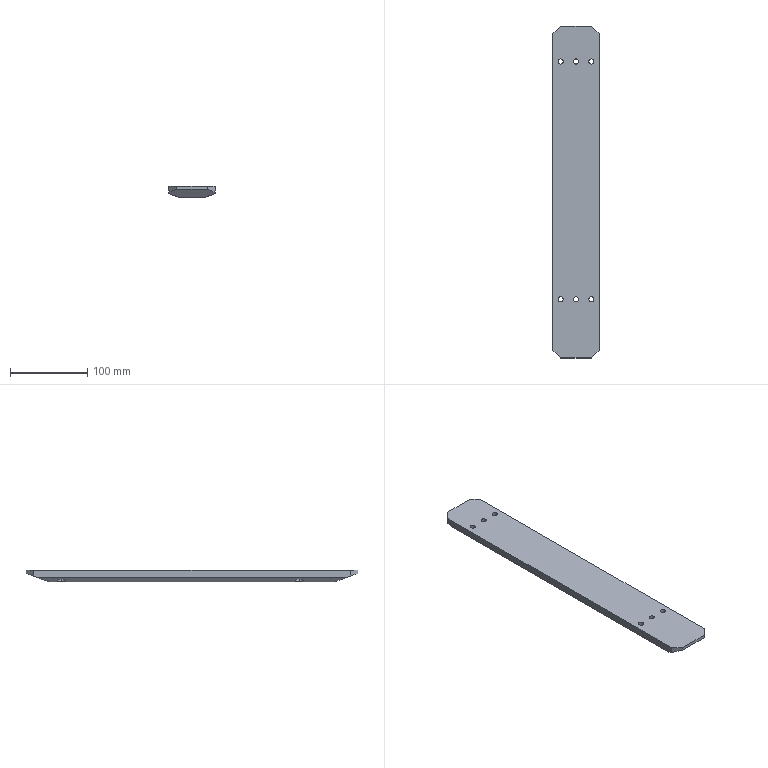Part | SolidWorks | features BaseBody 1 | 1 solid | 44 faces | box 60 x 430 x 15 mm | volume 329496 mm3 | cylinder 24 | plane 20 | commonest cylinder face diameters 6.6 x12 11 x12
STEP:
#1=CARTESIAN_POINT('',(25.5,169.,9.));
#2=VERTEX_POINT('',#1);
#3=CARTESIAN_POINT('',(14.5,169.,9.));
#4=VERTEX_POINT('',#3);
#5=CARTESIAN_POINT('',(20.,169.,9.));
#6=DIRECTION('',(0.,0.,-1.));
#7=DIRECTION('',(-1.,0.,0.));
#8=AXIS2_PLACEMENT_3D('',#5,#6,#7);
#9=CIRCLE('',#8,5.5);
#10=EDGE_CURVE('',#2,#4,#9,.T.);
#11=ORIENTED_EDGE('',*,*,#10,.F.);
#12=CARTESIAN_POINT('',(25.5,169.,3.822));
#13=VERTEX_POINT('',#12);
#14=CARTESIAN_POINT('',(25.5,169.,0.));
#15=DIRECTION('',(0.,0.,-1.));
#16=VECTOR('',#15,1000.);
#17=LINE('',#14,#16);
#18=EDGE_CURVE('',#2,#13,#17,.T.);
#19=ORIENTED_EDGE('',*,*,#18,.T.);
#20=CARTESIAN_POINT('',(15.,166.709,0.));
#21=VERTEX_POINT('',#20);
#22=CARTESIAN_POINT('',(25.5,169.,3.822));
#23=CARTESIAN_POINT('',(25.5,161.466,3.822));
#24=CARTESIAN_POINT('',(18.139,159.859,1.142));
#25=CARTESIAN_POINT('',(15.,166.709,0.));
#26=(BOUNDED_CURVE()B_SPLINE_CURVE(3,(#22,#23,#24,#25),.UNSPECIFIED.,.F.,.F.)B_SPLINE_CURVE_WITH_KNOTS((4,4),(3.142,5.853),.UNSPECIFIED.)CURVE()GEOMETRIC_REPRESENTATION_ITEM()RATIONAL_B_SPLINE_CURVE((1.,0.4755,0.4755,1.))REPRESENTATION_ITEM(''));
#27=EDGE_CURVE('',#13,#21,#26,.T.);
#28=ORIENTED_EDGE('',*,*,#27,.T.);
#29=CARTESIAN_POINT('',(14.5,169.,0.));
#30=VERTEX_POINT('',#29);
#31=CARTESIAN_POINT('',(20.,169.,0.));
#32=DIRECTION('',(0.,0.,-1.));
#33=DIRECTION('',(-1.,0.,0.));
#34=AXIS2_PLACEMENT_3D('',#31,#32,#33);
#35=CIRCLE('',#34,5.5);
#36=EDGE_CURVE('',#21,#30,#35,.T.);
#37=ORIENTED_EDGE('',*,*,#36,.T.);
#38=CARTESIAN_POINT('',(14.5,169.,0.));
#39=DIRECTION('',(0.,0.,-1.));
#40=VECTOR('',#39,1000.);
#41=LINE('',#38,#40);
#42=EDGE_CURVE('',#4,#30,#41,.T.);
#43=ORIENTED_EDGE('',*,*,#42,.F.);
#44=EDGE_LOOP('',(#11,#19,#28,#37,#43));
#45=FACE_OUTER_BOUND('',#44,.T.);
#46=CARTESIAN_POINT('',(20.,169.,0.));
#47=DIRECTION('',(0.,0.,-1.));
#48=DIRECTION('',(-1.,0.,0.));
#49=AXIS2_PLACEMENT_3D('',#46,#47,#48);
#50=CYLINDRICAL_SURFACE('',#49,5.5);
#51=ADVANCED_FACE('',(#45),#50,.F.);
#52=CARTESIAN_POINT('',(23.3,169.,15.));
#53=VERTEX_POINT('',#52);
#54=CARTESIAN_POINT('',(16.7,169.,15.));
#55=VERTEX_POINT('',#54);
#56=CARTESIAN_POINT('',(20.,169.,15.));
#57=DIRECTION('',(0.,0.,-1.));
#58=DIRECTION('',(-1.,0.,0.));
#59=AXIS2_PLACEMENT_3D('',#56,#57,#58);
#60=CIRCLE('',#59,3.3);
#61=EDGE_CURVE('',#53,#55,#60,.T.);
#62=ORIENTED_EDGE('',*,*,#61,.F.);
#63=CARTESIAN_POINT('',(23.3,169.,9.));
#64=VERTEX_POINT('',#63);
#65=CARTESIAN_POINT('',(23.3,169.,0.));
#66=DIRECTION('',(0.,0.,-1.));
#67=VECTOR('',#66,1000.);
#68=LINE('',#65,#67);
#69=EDGE_CURVE('',#53,#64,#68,.T.);
#70=ORIENTED_EDGE('',*,*,#69,.T.);
#71=CARTESIAN_POINT('',(16.7,169.,9.));
#72=VERTEX_POINT('',#71);
#73=CARTESIAN_POINT('',(20.,169.,9.));
#74=DIRECTION('',(0.,0.,-1.));
#75=DIRECTION('',(-1.,0.,0.));
#76=AXIS2_PLACEMENT_3D('',#73,#74,#75);
#77=CIRCLE('',#76,3.3);
#78=EDGE_CURVE('',#64,#72,#77,.T.);
#79=ORIENTED_EDGE('',*,*,#78,.T.);
#80=CARTESIAN_POINT('',(16.7,169.,0.));
#81=DIRECTION('',(0.,0.,-1.));
#82=VECTOR('',#81,1000.);
#83=LINE('',#80,#82);
#84=EDGE_CURVE('',#55,#72,#83,.T.);
#85=ORIENTED_EDGE('',*,*,#84,.F.);
#86=EDGE_LOOP('',(#62,#70,#79,#85));
#87=FACE_OUTER_BOUND('',#86,.T.);
#88=CARTESIAN_POINT('',(20.,169.,0.));
#89=DIRECTION('',(0.,0.,-1.));
#90=DIRECTION('',(-1.,0.,0.));
#91=AXIS2_PLACEMENT_3D('',#88,#89,#90);
#92=CYLINDRICAL_SURFACE('',#91,3.3);
#93=ADVANCED_FACE('',(#87),#92,.F.);
#94=CARTESIAN_POINT('',(5.5,169.,9.));
#95=VERTEX_POINT('',#94);
#96=CARTESIAN_POINT('',(-5.5,169.,9.));
#97=VERTEX_POINT('',#96);
#98=CARTESIAN_POINT('',(0.,169.,9.));
#99=DIRECTION('',(0.,0.,-1.));
#100=DIRECTION('',(-1.,0.,0.));
#101=AXIS2_PLACEMENT_3D('',#98,#99,#100);
#102=CIRCLE('',#101,5.5);
#103=EDGE_CURVE('',#95,#97,#102,.T.);
#104=ORIENTED_EDGE('',*,*,#103,.F.);
#105=CARTESIAN_POINT('',(5.5,169.,0.));
#106=VERTEX_POINT('',#105);
#107=CARTESIAN_POINT('',(5.5,169.,0.));
#108=DIRECTION('',(0.,0.,-1.));
#109=VECTOR('',#108,1000.);
#110=LINE('',#107,#109);
#111=EDGE_CURVE('',#95,#106,#110,.T.);
#112=ORIENTED_EDGE('',*,*,#111,.T.);
#113=CARTESIAN_POINT('',(-5.5,169.,0.));
#114=VERTEX_POINT('',#113);
#115=CARTESIAN_POINT('',(0.,169.,0.));
#116=DIRECTION('',(0.,0.,-1.));
#117=DIRECTION('',(-1.,0.,0.));
#118=AXIS2_PLACEMENT_3D('',#115,#116,#117);
#119=CIRCLE('',#118,5.5);
#120=EDGE_CURVE('',#106,#114,#119,.T.);
#121=ORIENTED_EDGE('',*,*,#120,.T.);
#122=CARTESIAN_POINT('',(-5.5,169.,0.));
#123=DIRECTION('',(0.,0.,-1.));
#124=VECTOR('',#123,1000.);
#125=LINE('',#122,#124);
#126=EDGE_CURVE('',#97,#114,#125,.T.);
#127=ORIENTED_EDGE('',*,*,#126,.F.);
#128=EDGE_LOOP('',(#104,#112,#121,#127));
#129=FACE_OUTER_BOUND('',#128,.T.);
#130=CARTESIAN_POINT('',(0.,169.,0.));
#131=DIRECTION('',(0.,0.,-1.));
#132=DIRECTION('',(-1.,0.,0.));
#133=AXIS2_PLACEMENT_3D('',#130,#131,#132);
#134=CYLINDRICAL_SURFACE('',#133,5.5);
#135=ADVANCED_FACE('',(#129),#134,.F.);
#136=CARTESIAN_POINT('',(3.3,169.,15.));
#137=VERTEX_POINT('',#136);
#138=CARTESIAN_POINT('',(-3.3,169.,15.));
#139=VERTEX_POINT('',#138);
#140=CARTESIAN_POINT('',(0.,169.,15.));
#141=DIRECTION('',(0.,0.,-1.));
#142=DIRECTION('',(-1.,0.,0.));
#143=AXIS2_PLACEMENT_3D('',#140,#141,#142);
#144=CIRCLE('',#143,3.3);
#145=EDGE_CURVE('',#137,#139,#144,.T.);
#146=ORIENTED_EDGE('',*,*,#145,.F.);
#147=CARTESIAN_POINT('',(3.3,169.,9.));
#148=VERTEX_POINT('',#147);
#149=CARTESIAN_POINT('',(3.3,169.,0.));
#150=DIRECTION('',(0.,0.,-1.));
#151=VECTOR('',#150,1000.);
#152=LINE('',#149,#151);
#153=EDGE_CURVE('',#137,#148,#152,.T.);
#154=ORIENTED_EDGE('',*,*,#153,.T.);
#155=CARTESIAN_POINT('',(-3.3,169.,9.));
#156=VERTEX_POINT('',#155);
#157=CARTESIAN_POINT('',(0.,169.,9.));
#158=DIRECTION('',(0.,0.,-1.));
#159=DIRECTION('',(-1.,0.,0.));
#160=AXIS2_PLACEMENT_3D('',#157,#158,#159);
#161=CIRCLE('',#160,3.3);
#162=EDGE_CURVE('',#148,#156,#161,.T.);
#163=ORIENTED_EDGE('',*,*,#162,.T.);
#164=CARTESIAN_POINT('',(-3.3,169.,0.));
#165=DIRECTION('',(0.,0.,-1.));
#166=VECTOR('',#165,1000.);
#167=LINE('',#164,#166);
#168=EDGE_CURVE('',#139,#156,#167,.T.);
#169=ORIENTED_EDGE('',*,*,#168,.F.);
#170=EDGE_LOOP('',(#146,#154,#163,#169));
#171=FACE_OUTER_BOUND('',#170,.T.);
#172=CARTESIAN_POINT('',(0.,169.,0.));
#173=DIRECTION('',(0.,0.,-1.));
#174=DIRECTION('',(-1.,0.,0.));
#175=AXIS2_PLACEMENT_3D('',#172,#173,#174);
#176=CYLINDRICAL_SURFACE('',#175,3.3);
#177=ADVANCED_FACE('',(#171),#176,.F.);
#178=CARTESIAN_POINT('',(-14.5,169.,9.));
#179=VERTEX_POINT('',#178);
#180=CARTESIAN_POINT('',(-25.5,169.,9.));
#181=VERTEX_POINT('',#180);
#182=CARTESIAN_POINT('',(-20.,169.,9.));
#183=DIRECTION('',(0.,0.,-1.));
#184=DIRECTION('',(-1.,0.,0.));
#185=AXIS2_PLACEMENT_3D('',#182,#183,#184);
#186=CIRCLE('',#185,5.5);
#187=EDGE_CURVE('',#179,#181,#186,.T.);
#188=ORIENTED_EDGE('',*,*,#187,.F.);
#189=CARTESIAN_POINT('',(-14.5,169.,0.));
#190=VERTEX_POINT('',#189);
#191=CARTESIAN_POINT('',(-14.5,169.,0.));
#192=DIRECTION('',(0.,0.,-1.));
#193=VECTOR('',#192,1000.);
#194=LINE('',#191,#193);
#195=EDGE_CURVE('',#179,#190,#194,.T.);
#196=ORIENTED_EDGE('',*,*,#195,.T.);
#197=CARTESIAN_POINT('',(-15.,166.709,0.));
#198=VERTEX_POINT('',#197);
#199=CARTESIAN_POINT('',(-20.,169.,0.));
#200=DIRECTION('',(0.,0.,-1.));
#201=DIRECTION('',(-1.,0.,0.));
#202=AXIS2_PLACEMENT_3D('',#199,#200,#201);
#203=CIRCLE('',#202,5.5);
#204=EDGE_CURVE('',#190,#198,#203,.T.);
#205=ORIENTED_EDGE('',*,*,#204,.T.);
#206=CARTESIAN_POINT('',(-25.5,169.,3.822));
#207=VERTEX_POINT('',#206);
#208=CARTESIAN_POINT('',(-15.,166.709,0.));
#209=CARTESIAN_POINT('',(-18.139,159.859,1.142));
#210=CARTESIAN_POINT('',(-25.5,161.466,3.822));
#211=CARTESIAN_POINT('',(-25.5,169.,3.822));
#212=(BOUNDED_CURVE()B_SPLINE_CURVE(3,(#208,#209,#210,#211),.UNSPECIFIED.,.F.,.F.)B_SPLINE_CURVE_WITH_KNOTS((4,4),(0.4297,3.142),.UNSPECIFIED.)CURVE()GEOMETRIC_REPRESENTATION_ITEM()RATIONAL_B_SPLINE_CURVE((1.,0.4755,0.4755,1.))REPRESENTATION_ITEM(''));
#213=EDGE_CURVE('',#198,#207,#212,.T.);
#214=ORIENTED_EDGE('',*,*,#213,.T.);
#215=CARTESIAN_POINT('',(-25.5,169.,0.));
#216=DIRECTION('',(0.,0.,-1.));
#217=VECTOR('',#216,1000.);
#218=LINE('',#215,#217);
#219=EDGE_CURVE('',#181,#207,#218,.T.);
#220=ORIENTED_EDGE('',*,*,#219,.F.);
#221=EDGE_LOOP('',(#188,#196,#205,#214,#220));
#222=FACE_OUTER_BOUND('',#221,.T.);
#223=CARTESIAN_POINT('',(-20.,169.,0.));
#224=DIRECTION('',(0.,0.,-1.));
#225=DIRECTION('',(-1.,0.,0.));
#226=AXIS2_PLACEMENT_3D('',#223,#224,#225);
#227=CYLINDRICAL_SURFACE('',#226,5.5);
#228=ADVANCED_FACE('',(#222),#227,.F.);
#229=CARTESIAN_POINT('',(-16.7,169.,15.));
#230=VERTEX_POINT('',#229);
#231=CARTESIAN_POINT('',(-23.3,169.,15.));
#232=VERTEX_POINT('',#231);
#233=CARTESIAN_POINT('',(-20.,169.,15.));
#234=DIRECTION('',(0.,0.,-1.));
#235=DIRECTION('',(-1.,0.,0.));
#236=AXIS2_PLACEMENT_3D('',#233,#234,#235);
#237=CIRCLE('',#236,3.3);
#238=EDGE_CURVE('',#230,#232,#237,.T.);
#239=ORIENTED_EDGE('',*,*,#238,.F.);
#240=CARTESIAN_POINT('',(-16.7,169.,9.));
#241=VERTEX_POINT('',#240);
#242=CARTESIAN_POINT('',(-16.7,169.,0.));
#243=DIRECTION('',(0.,0.,-1.));
#244=VECTOR('',#243,1000.);
#245=LINE('',#242,#244);
#246=EDGE_CURVE('',#230,#241,#245,.T.);
#247=ORIENTED_EDGE('',*,*,#246,.T.);
#248=CARTESIAN_POINT('',(-23.3,169.,9.));
#249=VERTEX_POINT('',#248);
#250=CARTESIAN_POINT('',(-20.,169.,9.));
#251=DIRECTION('',(0.,0.,-1.));
#252=DIRECTION('',(-1.,0.,0.));
#253=AXIS2_PLACEMENT_3D('',#250,#251,#252);
#254=CIRCLE('',#253,3.3);
#255=EDGE_CURVE('',#241,#249,#254,.T.);
#256=ORIENTED_EDGE('',*,*,#255,.T.);
#257=CARTESIAN_POINT('',(-23.3,169.,0.));
#258=DIRECTION('',(0.,0.,-1.));
#259=VECTOR('',#258,1000.);
#260=LINE('',#257,#259);
#261=EDGE_CURVE('',#232,#249,#260,.T.);
#262=ORIENTED_EDGE('',*,*,#261,.F.);
#263=EDGE_LOOP('',(#239,#247,#256,#262));
#264=FACE_OUTER_BOUND('',#263,.T.);
#265=CARTESIAN_POINT('',(-20.,169.,0.));
#266=DIRECTION('',(0.,0.,-1.));
#267=DIRECTION('',(-1.,0.,0.));
#268=AXIS2_PLACEMENT_3D('',#265,#266,#267);
#269=CYLINDRICAL_SURFACE('',#268,3.3);
#270=ADVANCED_FACE('',(#264),#269,.F.);
#271=CARTESIAN_POINT('',(25.5,-139.,9.));
#272=VERTEX_POINT('',#271);
#273=CARTESIAN_POINT('',(14.5,-139.,9.));
#274=VERTEX_POINT('',#273);
#275=CARTESIAN_POINT('',(20.,-139.,9.));
#276=DIRECTION('',(0.,0.,-1.));
#277=DIRECTION('',(-1.,0.,0.));
#278=AXIS2_PLACEMENT_3D('',#275,#276,#277);
#279=CIRCLE('',#278,5.5);
#280=EDGE_CURVE('',#272,#274,#279,.T.);
#281=ORIENTED_EDGE('',*,*,#280,.F.);
#282=CARTESIAN_POINT('',(25.5,-139.,3.822));
#283=VERTEX_POINT('',#282);
#284=CARTESIAN_POINT('',(25.5,-139.,0.));
#285=DIRECTION('',(0.,0.,-1.));
#286=VECTOR('',#285,1000.);
#287=LINE('',#284,#286);
#288=EDGE_CURVE('',#272,#283,#287,.T.);
#289=ORIENTED_EDGE('',*,*,#288,.T.);
#290=CARTESIAN_POINT('',(15.,-141.291,0.));
#291=VERTEX_POINT('',#290);
#292=CARTESIAN_POINT('',(25.5,-139.,3.822));
#293=CARTESIAN_POINT('',(25.5,-146.534,3.822));
#294=CARTESIAN_POINT('',(18.139,-148.141,1.142));
#295=CARTESIAN_POINT('',(15.,-141.291,0.));
#296=(BOUNDED_CURVE()B_SPLINE_CURVE(3,(#292,#293,#294,#295),.UNSPECIFIED.,.F.,.T.)B_SPLINE_CURVE_WITH_KNOTS((4,4),(3.142,5.853),.UNSPECIFIED.)CURVE()GEOMETRIC_REPRESENTATION_ITEM()RATIONAL_B_SPLINE_CURVE((1.,0.4755,0.4755,1.))REPRESENTATION_ITEM(''));
#297=EDGE_CURVE('',#283,#291,#296,.T.);
#298=ORIENTED_EDGE('',*,*,#297,.T.);
#299=CARTESIAN_POINT('',(14.5,-139.,0.));
#300=VERTEX_POINT('',#299);
#301=CARTESIAN_POINT('',(20.,-139.,0.));
#302=DIRECTION('',(0.,0.,-1.));
#303=DIRECTION('',(-1.,0.,0.));
#304=AXIS2_PLACEMENT_3D('',#301,#302,#303);
#305=CIRCLE('',#304,5.5);
#306=EDGE_CURVE('',#291,#300,#305,.T.);
#307=ORIENTED_EDGE('',*,*,#306,.T.);
#308=CARTESIAN_POINT('',(14.5,-139.,0.));
#309=DIRECTION('',(0.,0.,-1.));
#310=VECTOR('',#309,1000.);
#311=LINE('',#308,#310);
#312=EDGE_CURVE('',#274,#300,#311,.T.);
#313=ORIENTED_EDGE('',*,*,#312,.F.);
#314=EDGE_LOOP('',(#281,#289,#298,#307,#313));
#315=FACE_OUTER_BOUND('',#314,.T.);
#316=CARTESIAN_POINT('',(20.,-139.,0.));
#317=DIRECTION('',(0.,0.,-1.));
#318=DIRECTION('',(-1.,0.,0.));
#319=AXIS2_PLACEMENT_3D('',#316,#317,#318);
#320=CYLINDRICAL_SURFACE('',#319,5.5);
#321=ADVANCED_FACE('',(#315),#320,.F.);
#322=CARTESIAN_POINT('',(23.3,-139.,15.));
#323=VERTEX_POINT('',#322);
#324=CARTESIAN_POINT('',(16.7,-139.,15.));
#325=VERTEX_POINT('',#324);
#326=CARTESIAN_POINT('',(20.,-139.,15.));
#327=DIRECTION('',(0.,0.,-1.));
#328=DIRECTION('',(-1.,0.,0.));
#329=AXIS2_PLACEMENT_3D('',#326,#327,#328);
#330=CIRCLE('',#329,3.3);
#331=EDGE_CURVE('',#323,#325,#330,.T.);
#332=ORIENTED_EDGE('',*,*,#331,.F.);
#333=CARTESIAN_POINT('',(23.3,-139.,9.));
#334=VERTEX_POINT('',#333);
#335=CARTESIAN_POINT('',(23.3,-139.,0.));
#336=DIRECTION('',(0.,0.,-1.));
#337=VECTOR('',#336,1000.);
#338=LINE('',#335,#337);
#339=EDGE_CURVE('',#323,#334,#338,.T.);
#340=ORIENTED_EDGE('',*,*,#339,.T.);
#341=CARTESIAN_POINT('',(16.7,-139.,9.));
#342=VERTEX_POINT('',#341);
#343=CARTESIAN_POINT('',(20.,-139.,9.));
#344=DIRECTION('',(0.,0.,-1.));
#345=DIRECTION('',(-1.,0.,0.));
#346=AXIS2_PLACEMENT_3D('',#343,#344,#345);
#347=CIRCLE('',#346,3.3);
#348=EDGE_CURVE('',#334,#342,#347,.T.);
#349=ORIENTED_EDGE('',*,*,#348,.T.);
#350=CARTESIAN_POINT('',(16.7,-139.,0.));
#351=DIRECTION('',(0.,0.,-1.));
#352=VECTOR('',#351,1000.);
#353=LINE('',#350,#352);
#354=EDGE_CURVE('',#325,#342,#353,.T.);
#355=ORIENTED_EDGE('',*,*,#354,.F.);
#356=EDGE_LOOP('',(#332,#340,#349,#355));
#357=FACE_OUTER_BOUND('',#356,.T.);
#358=CARTESIAN_POINT('',(20.,-139.,0.));
#359=DIRECTION('',(0.,0.,-1.));
#360=DIRECTION('',(-1.,0.,0.));
#361=AXIS2_PLACEMENT_3D('',#358,#359,#360);
#362=CYLINDRICAL_SURFACE('',#361,3.3);
#363=ADVANCED_FACE('',(#357),#362,.F.);
#364=CARTESIAN_POINT('',(5.5,-139.,9.));
#365=VERTEX_POINT('',#364);
#366=CARTESIAN_POINT('',(-5.5,-139.,9.));
#367=VERTEX_POINT('',#366);
#368=CARTESIAN_POINT('',(0.,-139.,9.));
#369=DIRECTION('',(0.,0.,-1.));
#370=DIRECTION('',(-1.,0.,0.));
#371=AXIS2_PLACEMENT_3D('',#368,#369,#370);
#372=CIRCLE('',#371,5.5);
#373=EDGE_CURVE('',#365,#367,#372,.T.);
#374=ORIENTED_EDGE('',*,*,#373,.F.);
#375=CARTESIAN_POINT('',(5.5,-139.,0.));
#376=VERTEX_POINT('',#375);
#377=CARTESIAN_POINT('',(5.5,-139.,0.));
#378=DIRECTION('',(0.,0.,-1.));
#379=VECTOR('',#378,1000.);
#380=LINE('',#377,#379);
#381=EDGE_CURVE('',#365,#376,#380,.T.);
#382=ORIENTED_EDGE('',*,*,#381,.T.);
#383=CARTESIAN_POINT('',(-5.5,-139.,0.));
#384=VERTEX_POINT('',#383);
#385=CARTESIAN_POINT('',(0.,-139.,0.));
#386=DIRECTION('',(0.,0.,-1.));
#387=DIRECTION('',(-1.,0.,0.));
#388=AXIS2_PLACEMENT_3D('',#385,#386,#387);
#389=CIRCLE('',#388,5.5);
#390=EDGE_CURVE('',#376,#384,#389,.T.);
#391=ORIENTED_EDGE('',*,*,#390,.T.);
#392=CARTESIAN_POINT('',(-5.5,-139.,0.));
#393=DIRECTION('',(0.,0.,-1.));
#394=VECTOR('',#393,1000.);
#395=LINE('',#392,#394);
#396=EDGE_CURVE('',#367,#384,#395,.T.);
#397=ORIENTED_EDGE('',*,*,#396,.F.);
#398=EDGE_LOOP('',(#374,#382,#391,#397));
#399=FACE_OUTER_BOUND('',#398,.T.);
#400=CARTESIAN_POINT('',(0.,-139.,0.));
#401=DIRECTION('',(0.,0.,-1.));
#402=DIRECTION('',(-1.,0.,0.));
#403=AXIS2_PLACEMENT_3D('',#400,#401,#402);
#404=CYLINDRICAL_SURFACE('',#403,5.5);
#405=ADVANCED_FACE('',(#399),#404,.F.);
#406=CARTESIAN_POINT('',(3.3,-139.,15.));
#407=VERTEX_POINT('',#406);
#408=CARTESIAN_POINT('',(-3.3,-139.,15.));
#409=VERTEX_POINT('',#408);
#410=CARTESIAN_POINT('',(0.,-139.,15.));
#411=DIRECTION('',(0.,0.,-1.));
#412=DIRECTION('',(-1.,0.,0.));
#413=AXIS2_PLACEMENT_3D('',#410,#411,#412);
#414=CIRCLE('',#413,3.3);
#415=EDGE_CURVE('',#407,#409,#414,.T.);
#416=ORIENTED_EDGE('',*,*,#415,.F.);
#417=CARTESIAN_POINT('',(3.3,-139.,9.));
#418=VERTEX_POINT('',#417);
#419=CARTESIAN_POINT('',(3.3,-139.,0.));
#420=DIRECTION('',(0.,0.,-1.));
#421=VECTOR('',#420,1000.);
#422=LINE('',#419,#421);
#423=EDGE_CURVE('',#407,#418,#422,.T.);
#424=ORIENTED_EDGE('',*,*,#423,.T.);
#425=CARTESIAN_POINT('',(-3.3,-139.,9.));
#426=VERTEX_POINT('',#425);
#427=CARTESIAN_POINT('',(0.,-139.,9.));
#428=DIRECTION('',(0.,0.,-1.));
#429=DIRECTION('',(-1.,0.,0.));
#430=AXIS2_PLACEMENT_3D('',#427,#428,#429);
#431=CIRCLE('',#430,3.3);
#432=EDGE_CURVE('',#418,#426,#431,.T.);
#433=ORIENTED_EDGE('',*,*,#432,.T.);
#434=CARTESIAN_POINT('',(-3.3,-139.,0.));
#435=DIRECTION('',(0.,0.,-1.));
#436=VECTOR('',#435,1000.);
#437=LINE('',#434,#436);
#438=EDGE_CURVE('',#409,#426,#437,.T.);
#439=ORIENTED_EDGE('',*,*,#438,.F.);
#440=EDGE_LOOP('',(#416,#424,#433,#439));
#441=FACE_OUTER_BOUND('',#440,.T.);
#442=CARTESIAN_POINT('',(0.,-139.,0.));
#443=DIRECTION('',(0.,0.,-1.));
#444=DIRECTION('',(-1.,0.,0.));
#445=AXIS2_PLACEMENT_3D('',#442,#443,#444);
#446=CYLINDRICAL_SURFACE('',#445,3.3);
#447=ADVANCED_FACE('',(#441),#446,.F.);
#448=CARTESIAN_POINT('',(-14.5,-139.,9.));
#449=VERTEX_POINT('',#448);
#450=CARTESIAN_POINT('',(-25.5,-139.,9.));
#451=VERTEX_POINT('',#450);
#452=CARTESIAN_POINT('',(-20.,-139.,9.));
#453=DIRECTION('',(0.,0.,-1.));
#454=DIRECTION('',(-1.,0.,0.));
#455=AXIS2_PLACEMENT_3D('',#452,#453,#454);
#456=CIRCLE('',#455,5.5);
#457=EDGE_CURVE('',#449,#451,#456,.T.);
#458=ORIENTED_EDGE('',*,*,#457,.F.);
#459=CARTESIAN_POINT('',(-14.5,-139.,0.));
#460=VERTEX_POINT('',#459);
#461=CARTESIAN_POINT('',(-14.5,-139.,0.));
#462=DIRECTION('',(0.,0.,-1.));
#463=VECTOR('',#462,1000.);
#464=LINE('',#461,#463);
#465=EDGE_CURVE('',#449,#460,#464,.T.);
#466=ORIENTED_EDGE('',*,*,#465,.T.);
#467=CARTESIAN_POINT('',(-15.,-141.291,0.));
#468=VERTEX_POINT('',#467);
#469=CARTESIAN_POINT('',(-20.,-139.,0.));
#470=DIRECTION('',(0.,0.,-1.));
#471=DIRECTION('',(-1.,0.,0.));
#472=AXIS2_PLACEMENT_3D('',#469,#470,#471);
#473=CIRCLE('',#472,5.5);
#474=EDGE_CURVE('',#460,#468,#473,.T.);
#475=ORIENTED_EDGE('',*,*,#474,.T.);
#476=CARTESIAN_POINT('',(-25.5,-139.,3.822));
#477=VERTEX_POINT('',#476);
#478=CARTESIAN_POINT('',(-15.,-141.291,0.));
#479=CARTESIAN_POINT('',(-18.139,-148.141,1.142));
#480=CARTESIAN_POINT('',(-25.5,-146.534,3.822));
#481=CARTESIAN_POINT('',(-25.5,-139.,3.822));
#482=(BOUNDED_CURVE()B_SPLINE_CURVE(3,(#478,#479,#480,#481),.UNSPECIFIED.,.F.,.T.)B_SPLINE_CURVE_WITH_KNOTS((4,4),(0.4297,3.142),.UNSPECIFIED.)CURVE()GEOMETRIC_REPRESENTATION_ITEM()RATIONAL_B_SPLINE_CURVE((1.,0.4755,0.4755,1.))REPRESENTATION_ITEM(''));
#483=EDGE_CURVE('',#468,#477,#482,.T.);
#484=ORIENTED_EDGE('',*,*,#483,.T.);
#485=CARTESIAN_POINT('',(-25.5,-139.,0.));
#486=DIRECTION('',(0.,0.,-1.));
#487=VECTOR('',#486,1000.);
#488=LINE('',#485,#487);
#489=EDGE_CURVE('',#451,#477,#488,.T.);
#490=ORIENTED_EDGE('',*,*,#489,.F.);
#491=EDGE_LOOP('',(#458,#466,#475,#484,#490));
#492=FACE_OUTER_BOUND('',#491,.T.);
#493=CARTESIAN_POINT('',(-20.,-139.,0.));
#494=DIRECTION('',(0.,0.,-1.));
#495=DIRECTION('',(-1.,0.,0.));
#496=AXIS2_PLACEMENT_3D('',#493,#494,#495);
#497=CYLINDRICAL_SURFACE('',#496,5.5);
#498=ADVANCED_FACE('',(#492),#497,.F.);
#499=CARTESIAN_POINT('',(-16.7,-139.,15.));
#500=VERTEX_POINT('',#499);
#501=CARTESIAN_POINT('',(-23.3,-139.,15.));
#502=VERTEX_POINT('',#501);
#503=CARTESIAN_POINT('',(-20.,-139.,15.));
#504=DIRECTION('',(0.,0.,-1.));
#505=DIRECTION('',(-1.,0.,0.));
#506=AXIS2_PLACEMENT_3D('',#503,#504,#505);
#507=CIRCLE('',#506,3.3);
#508=EDGE_CURVE('',#500,#502,#507,.T.);
#509=ORIENTED_EDGE('',*,*,#508,.F.);
#510=CARTESIAN_POINT('',(-16.7,-139.,9.));
#511=VERTEX_POINT('',#510);
#512=CARTESIAN_POINT('',(-16.7,-139.,0.));
#513=DIRECTION('',(0.,0.,-1.));
#514=VECTOR('',#513,1000.);
#515=LINE('',#512,#514);
#516=EDGE_CURVE('',#500,#511,#515,.T.);
#517=ORIENTED_EDGE('',*,*,#516,.T.);
#518=CARTESIAN_POINT('',(-23.3,-139.,9.));
#519=VERTEX_POINT('',#518);
#520=CARTESIAN_POINT('',(-20.,-139.,9.));
#521=DIRECTION('',(0.,0.,-1.));
#522=DIRECTION('',(-1.,0.,0.));
#523=AXIS2_PLACEMENT_3D('',#520,#521,#522);
#524=CIRCLE('',#523,3.3);
#525=EDGE_CURVE('',#511,#519,#524,.T.);
#526=ORIENTED_EDGE('',*,*,#525,.T.);
#527=CARTESIAN_POINT('',(-23.3,-139.,0.));
#528=DIRECTION('',(0.,0.,-1.));
#529=VECTOR('',#528,1000.);
#530=LINE('',#527,#529);
#531=EDGE_CURVE('',#502,#519,#530,.T.);
#532=ORIENTED_EDGE('',*,*,#531,.F.);
#533=EDGE_LOOP('',(#509,#517,#526,#532));
#534=FACE_OUTER_BOUND('',#533,.T.);
#535=CARTESIAN_POINT('',(-20.,-139.,0.));
#536=DIRECTION('',(0.,0.,-1.));
#537=DIRECTION('',(-1.,0.,0.));
#538=AXIS2_PLACEMENT_3D('',#535,#536,#537);
#539=CYLINDRICAL_SURFACE('',#538,3.3);
#540=ADVANCED_FACE('',(#534),#539,.F.);
#541=CARTESIAN_POINT('',(30.,-205.,7.279));
#542=VERTEX_POINT('',#541);
#543=CARTESIAN_POINT('',(30.,-200.,5.46));
#544=VERTEX_POINT('',#543);
#545=CARTESIAN_POINT('',(30.,-215.,10.919));
#546=DIRECTION('',(0.,0.9397,-0.342));
#547=VECTOR('',#546,1000.);
#548=LINE('',#545,#547);
#549=EDGE_CURVE('',#542,#544,#548,.T.);
#550=ORIENTED_EDGE('',*,*,#549,.T.);
#551=CARTESIAN_POINT('',(30.,200.,5.46));
#552=VERTEX_POINT('',#551);
#553=CARTESIAN_POINT('',(30.,215.,5.46));
#554=DIRECTION('',(0.,1.,0.));
#555=VECTOR('',#554,1000.);
#556=LINE('',#553,#555);
#557=EDGE_CURVE('',#544,#552,#556,.T.);
#558=ORIENTED_EDGE('',*,*,#557,.T.);
#559=CARTESIAN_POINT('',(30.,205.,7.279));
#560=VERTEX_POINT('',#559);
#561=CARTESIAN_POINT('',(30.,215.,10.919));
#562=DIRECTION('',(0.,0.9397,0.342));
#563=VECTOR('',#562,1000.);
#564=LINE('',#561,#563);
#565=EDGE_CURVE('',#552,#560,#564,.T.);
#566=ORIENTED_EDGE('',*,*,#565,.T.);
#567=CARTESIAN_POINT('',(30.,205.,15.));
#568=VERTEX_POINT('',#567);
#569=CARTESIAN_POINT('',(30.,205.,15.));
#570=DIRECTION('',(0.,0.,1.));
#571=VECTOR('',#570,1000.);
#572=LINE('',#569,#571);
#573=EDGE_CURVE('',#560,#568,#572,.T.);
#574=ORIENTED_EDGE('',*,*,#573,.T.);
#575=CARTESIAN_POINT('',(30.,-205.,15.));
#576=VERTEX_POINT('',#575);
#577=CARTESIAN_POINT('',(30.,215.,15.));
#578=DIRECTION('',(0.,1.,0.));
#579=VECTOR('',#578,1000.);
#580=LINE('',#577,#579);
#581=EDGE_CURVE('',#576,#568,#580,.T.);
#582=ORIENTED_EDGE('',*,*,#581,.F.);
#583=CARTESIAN_POINT('',(30.,-205.,15.));
#584=DIRECTION('',(0.,0.,-1.));
#585=VECTOR('',#584,1000.);
#586=LINE('',#583,#585);
#587=EDGE_CURVE('',#576,#542,#586,.T.);
#588=ORIENTED_EDGE('',*,*,#587,.T.);
#589=EDGE_LOOP('',(#550,#558,#566,#574,#582,#588));
#590=FACE_OUTER_BOUND('',#589,.T.);
#591=CARTESIAN_POINT('',(30.,215.,15.));
#592=DIRECTION('',(-1.,0.,0.));
#593=DIRECTION('',(0.,-1.,0.));
#594=AXIS2_PLACEMENT_3D('',#591,#592,#593);
#595=PLANE('',#594);
#596=ADVANCED_FACE('',(#590),#595,.F.);
#597=CARTESIAN_POINT('',(20.,215.,15.));
#598=VERTEX_POINT('',#597);
#599=CARTESIAN_POINT('',(20.,215.,10.919));
#600=VERTEX_POINT('',#599);
#601=CARTESIAN_POINT('',(20.,215.,15.));
#602=DIRECTION('',(0.,0.,-1.));
#603=VECTOR('',#602,1000.);
#604=LINE('',#601,#603);
#605=EDGE_CURVE('',#598,#600,#604,.T.);
#606=ORIENTED_EDGE('',*,*,#605,.T.);
#607=CARTESIAN_POINT('',(-20.,215.,10.919));
#608=VERTEX_POINT('',#607);
#609=CARTESIAN_POINT('',(-30.,215.,10.919));
#610=DIRECTION('',(-1.,0.,0.));
#611=VECTOR('',#610,1000.);
#612=LINE('',#609,#611);
#613=EDGE_CURVE('',#600,#608,#612,.T.);
#614=ORIENTED_EDGE('',*,*,#613,.T.);
#615=CARTESIAN_POINT('',(-20.,215.,15.));
#616=VERTEX_POINT('',#615);
#617=CARTESIAN_POINT('',(-20.,215.,15.));
#618=DIRECTION('',(0.,0.,1.));
#619=VECTOR('',#618,1000.);
#620=LINE('',#617,#619);
#621=EDGE_CURVE('',#608,#616,#620,.T.);
#622=ORIENTED_EDGE('',*,*,#621,.T.);
#623=CARTESIAN_POINT('',(-30.,215.,15.));
#624=DIRECTION('',(-1.,0.,0.));
#625=VECTOR('',#624,1000.);
#626=LINE('',#623,#625);
#627=EDGE_CURVE('',#598,#616,#626,.T.);
#628=ORIENTED_EDGE('',*,*,#627,.F.);
#629=EDGE_LOOP('',(#606,#614,#622,#628));
#630=FACE_OUTER_BOUND('',#629,.T.);
#631=CARTESIAN_POINT('',(-30.,215.,15.));
#632=DIRECTION('',(0.,-1.,0.));
#633=DIRECTION('',(0.,0.,-1.));
#634=AXIS2_PLACEMENT_3D('',#631,#632,#633);
#635=PLANE('',#634);
#636=ADVANCED_FACE('',(#630),#635,.F.);
#637=CARTESIAN_POINT('',(-30.,205.,7.279));
#638=VERTEX_POINT('',#637);
#639=CARTESIAN_POINT('',(-30.,200.,5.46));
#640=VERTEX_POINT('',#639);
#641=CARTESIAN_POINT('',(-30.,215.,10.919));
#642=DIRECTION('',(0.,-0.9397,-0.342));
#643=VECTOR('',#642,1000.);
#644=LINE('',#641,#643);
#645=EDGE_CURVE('',#638,#640,#644,.T.);
#646=ORIENTED_EDGE('',*,*,#645,.T.);
#647=CARTESIAN_POINT('',(-30.,-200.,5.46));
#648=VERTEX_POINT('',#647);
#649=CARTESIAN_POINT('',(-30.,215.,5.46));
#650=DIRECTION('',(0.,-1.,0.));
#651=VECTOR('',#650,1000.);
#652=LINE('',#649,#651);
#653=EDGE_CURVE('',#640,#648,#652,.T.);
#654=ORIENTED_EDGE('',*,*,#653,.T.);
#655=CARTESIAN_POINT('',(-30.,-205.,7.279));
#656=VERTEX_POINT('',#655);
#657=CARTESIAN_POINT('',(-30.,-215.,10.919));
#658=DIRECTION('',(0.,-0.9397,0.342));
#659=VECTOR('',#658,1000.);
#660=LINE('',#657,#659);
#661=EDGE_CURVE('',#648,#656,#660,.T.);
#662=ORIENTED_EDGE('',*,*,#661,.T.);
#663=CARTESIAN_POINT('',(-30.,-205.,15.));
#664=VERTEX_POINT('',#663);
#665=CARTESIAN_POINT('',(-30.,-205.,15.));
#666=DIRECTION('',(0.,0.,1.));
#667=VECTOR('',#666,1000.);
#668=LINE('',#665,#667);
#669=EDGE_CURVE('',#656,#664,#668,.T.);
#670=ORIENTED_EDGE('',*,*,#669,.T.);
#671=CARTESIAN_POINT('',(-30.,205.,15.));
#672=VERTEX_POINT('',#671);
#673=CARTESIAN_POINT('',(-30.,215.,15.));
#674=DIRECTION('',(0.,-1.,0.));
#675=VECTOR('',#674,1000.);
#676=LINE('',#673,#675);
#677=EDGE_CURVE('',#672,#664,#676,.T.);
#678=ORIENTED_EDGE('',*,*,#677,.F.);
#679=CARTESIAN_POINT('',(-30.,205.,15.));
#680=DIRECTION('',(0.,0.,-1.));
#681=VECTOR('',#680,1000.);
#682=LINE('',#679,#681);
#683=EDGE_CURVE('',#672,#638,#682,.T.);
#684=ORIENTED_EDGE('',*,*,#683,.T.);
#685=EDGE_LOOP('',(#646,#654,#662,#670,#678,#684));
#686=FACE_OUTER_BOUND('',#685,.T.);
#687=CARTESIAN_POINT('',(-30.,215.,15.));
#688=DIRECTION('',(1.,0.,0.));
#689=DIRECTION('',(0.,1.,0.));
#690=AXIS2_PLACEMENT_3D('',#687,#688,#689);
#691=PLANE('',#690);
#692=ADVANCED_FACE('',(#686),#691,.F.);
#693=CARTESIAN_POINT('',(-20.,-215.,15.));
#694=VERTEX_POINT('',#693);
#695=CARTESIAN_POINT('',(-20.,-215.,10.919));
#696=VERTEX_POINT('',#695);
#697=CARTESIAN_POINT('',(-20.,-215.,15.));
#698=DIRECTION('',(0.,0.,-1.));
#699=VECTOR('',#698,1000.);
#700=LINE('',#697,#699);
#701=EDGE_CURVE('',#694,#696,#700,.T.);
#702=ORIENTED_EDGE('',*,*,#701,.T.);
#703=CARTESIAN_POINT('',(20.,-215.,10.919));
#704=VERTEX_POINT('',#703);
#705=CARTESIAN_POINT('',(-30.,-215.,10.919));
#706=DIRECTION('',(1.,0.,0.));
#707=VECTOR('',#706,1000.);
#708=LINE('',#705,#707);
#709=EDGE_CURVE('',#696,#704,#708,.T.);
#710=ORIENTED_EDGE('',*,*,#709,.T.);
#711=CARTESIAN_POINT('',(20.,-215.,15.));
#712=VERTEX_POINT('',#711);
#713=CARTESIAN_POINT('',(20.,-215.,15.));
#714=DIRECTION('',(0.,0.,1.));
#715=VECTOR('',#714,1000.);
#716=LINE('',#713,#715);
#717=EDGE_CURVE('',#704,#712,#716,.T.);
#718=ORIENTED_EDGE('',*,*,#717,.T.);
#719=CARTESIAN_POINT('',(-30.,-215.,15.));
#720=DIRECTION('',(1.,0.,0.));
#721=VECTOR('',#720,1000.);
#722=LINE('',#719,#721);
#723=EDGE_CURVE('',#694,#712,#722,.T.);
#724=ORIENTED_EDGE('',*,*,#723,.F.);
#725=EDGE_LOOP('',(#702,#710,#718,#724));
#726=FACE_OUTER_BOUND('',#725,.T.);
#727=CARTESIAN_POINT('',(-30.,-215.,15.));
#728=DIRECTION('',(0.,1.,0.));
#729=DIRECTION('',(0.,0.,1.));
#730=AXIS2_PLACEMENT_3D('',#727,#728,#729);
#731=PLANE('',#730);
#732=ADVANCED_FACE('',(#726),#731,.F.);
#733=CARTESIAN_POINT('',(20.,169.,15.));
#734=DIRECTION('',(0.,0.,-1.));
#735=DIRECTION('',(-1.,0.,0.));
#736=AXIS2_PLACEMENT_3D('',#733,#734,#735);
#737=CIRCLE('',#736,3.3);
#738=EDGE_CURVE('',#55,#53,#737,.T.);
#739=ORIENTED_EDGE('',*,*,#738,.T.);
#740=ORIENTED_EDGE('',*,*,#61,.T.);
#741=EDGE_LOOP('',(#739,#740));
#742=FACE_BOUND('',#741,.T.);
#743=CARTESIAN_POINT('',(0.,169.,15.));
#744=DIRECTION('',(0.,0.,-1.));
#745=DIRECTION('',(-1.,0.,0.));
#746=AXIS2_PLACEMENT_3D('',#743,#744,#745);
#747=CIRCLE('',#746,3.3);
#748=EDGE_CURVE('',#139,#137,#747,.T.);
#749=ORIENTED_EDGE('',*,*,#748,.T.);
#750=ORIENTED_EDGE('',*,*,#145,.T.);
#751=EDGE_LOOP('',(#749,#750));
#752=FACE_BOUND('',#751,.T.);
#753=CARTESIAN_POINT('',(-20.,169.,15.));
#754=DIRECTION('',(0.,0.,-1.));
#755=DIRECTION('',(-1.,0.,0.));
#756=AXIS2_PLACEMENT_3D('',#753,#754,#755);
#757=CIRCLE('',#756,3.3);
#758=EDGE_CURVE('',#232,#230,#757,.T.);
#759=ORIENTED_EDGE('',*,*,#758,.T.);
#760=ORIENTED_EDGE('',*,*,#238,.T.);
#761=EDGE_LOOP('',(#759,#760));
#762=FACE_BOUND('',#761,.T.);
#763=CARTESIAN_POINT('',(20.,-139.,15.));
#764=DIRECTION('',(0.,0.,-1.));
#765=DIRECTION('',(-1.,0.,0.));
#766=AXIS2_PLACEMENT_3D('',#763,#764,#765);
#767=CIRCLE('',#766,3.3);
#768=EDGE_CURVE('',#325,#323,#767,.T.);
#769=ORIENTED_EDGE('',*,*,#768,.T.);
#770=ORIENTED_EDGE('',*,*,#331,.T.);
#771=EDGE_LOOP('',(#769,#770));
#772=FACE_BOUND('',#771,.T.);
#773=CARTESIAN_POINT('',(0.,-139.,15.));
#774=DIRECTION('',(0.,0.,-1.));
#775=DIRECTION('',(-1.,0.,0.));
#776=AXIS2_PLACEMENT_3D('',#773,#774,#775);
#777=CIRCLE('',#776,3.3);
#778=EDGE_CURVE('',#409,#407,#777,.T.);
#779=ORIENTED_EDGE('',*,*,#778,.T.);
#780=ORIENTED_EDGE('',*,*,#415,.T.);
#781=EDGE_LOOP('',(#779,#780));
#782=FACE_BOUND('',#781,.T.);
#783=CARTESIAN_POINT('',(-20.,-139.,15.));
#784=DIRECTION('',(0.,0.,-1.));
#785=DIRECTION('',(-1.,0.,0.));
#786=AXIS2_PLACEMENT_3D('',#783,#784,#785);
#787=CIRCLE('',#786,3.3);
#788=EDGE_CURVE('',#502,#500,#787,.T.);
#789=ORIENTED_EDGE('',*,*,#788,.T.);
#790=ORIENTED_EDGE('',*,*,#508,.T.);
#791=EDGE_LOOP('',(#789,#790));
#792=FACE_BOUND('',#791,.T.);
#793=ORIENTED_EDGE('',*,*,#723,.T.);
#794=CARTESIAN_POINT('',(117.5,-117.5,15.));
#795=DIRECTION('',(0.7071,0.7071,0.));
#796=VECTOR('',#795,1000.);
#797=LINE('',#794,#796);
#798=EDGE_CURVE('',#712,#576,#797,.T.);
#799=ORIENTED_EDGE('',*,*,#798,.T.);
#800=ORIENTED_EDGE('',*,*,#581,.T.);
#801=CARTESIAN_POINT('',(117.5,117.5,15.));
#802=DIRECTION('',(-0.7071,0.7071,0.));
#803=VECTOR('',#802,1000.);
#804=LINE('',#801,#803);
#805=EDGE_CURVE('',#568,#598,#804,.T.);
#806=ORIENTED_EDGE('',*,*,#805,.T.);
#807=ORIENTED_EDGE('',*,*,#627,.T.);
#808=CARTESIAN_POINT('',(-117.5,117.5,15.));
#809=DIRECTION('',(-0.7071,-0.7071,0.));
#810=VECTOR('',#809,1000.);
#811=LINE('',#808,#810);
#812=EDGE_CURVE('',#616,#672,#811,.T.);
#813=ORIENTED_EDGE('',*,*,#812,.T.);
#814=ORIENTED_EDGE('',*,*,#677,.T.);
#815=CARTESIAN_POINT('',(-117.5,-117.5,15.));
#816=DIRECTION('',(0.7071,-0.7071,0.));
#817=VECTOR('',#816,1000.);
#818=LINE('',#815,#817);
#819=EDGE_CURVE('',#664,#694,#818,.T.);
#820=ORIENTED_EDGE('',*,*,#819,.T.);
#821=EDGE_LOOP('',(#793,#799,#800,#806,#807,#813,#814,#820));
#822=FACE_OUTER_BOUND('',#821,.T.);
#823=CARTESIAN_POINT('',(0.,0.,15.));
#824=DIRECTION('',(0.,0.,1.));
#825=DIRECTION('',(1.,0.,0.));
#826=AXIS2_PLACEMENT_3D('',#823,#824,#825);
#827=PLANE('',#826);
#828=ADVANCED_FACE('',(#742,#752,#762,#772,#782,#792,#822),#827,.T.);
#829=CARTESIAN_POINT('',(0.,169.,0.));
#830=DIRECTION('',(0.,0.,-1.));
#831=DIRECTION('',(-1.,0.,0.));
#832=AXIS2_PLACEMENT_3D('',#829,#830,#831);
#833=CIRCLE('',#832,5.5);
#834=EDGE_CURVE('',#114,#106,#833,.T.);
#835=ORIENTED_EDGE('',*,*,#834,.F.);
#836=ORIENTED_EDGE('',*,*,#120,.F.);
#837=EDGE_LOOP('',(#835,#836));
#838=FACE_BOUND('',#837,.T.);
#839=CARTESIAN_POINT('',(0.,-139.,0.));
#840=DIRECTION('',(0.,0.,-1.));
#841=DIRECTION('',(-1.,0.,0.));
#842=AXIS2_PLACEMENT_3D('',#839,#840,#841);
#843=CIRCLE('',#842,5.5);
#844=EDGE_CURVE('',#384,#376,#843,.T.);
#845=ORIENTED_EDGE('',*,*,#844,.F.);
#846=ORIENTED_EDGE('',*,*,#390,.F.);
#847=EDGE_LOOP('',(#845,#846));
#848=FACE_BOUND('',#847,.T.);
#849=CARTESIAN_POINT('',(15.,185.,0.));
#850=VERTEX_POINT('',#849);
#851=CARTESIAN_POINT('',(15.,171.291,0.));
#852=VERTEX_POINT('',#851);
#853=CARTESIAN_POINT('',(15.,0.,0.));
#854=DIRECTION('',(0.,-1.,0.));
#855=VECTOR('',#854,1000.);
#856=LINE('',#853,#855);
#857=EDGE_CURVE('',#850,#852,#856,.T.);
#858=ORIENTED_EDGE('',*,*,#857,.T.);
#859=CARTESIAN_POINT('',(20.,169.,0.));
#860=DIRECTION('',(0.,0.,-1.));
#861=DIRECTION('',(-1.,0.,0.));
#862=AXIS2_PLACEMENT_3D('',#859,#860,#861);
#863=CIRCLE('',#862,5.5);
#864=EDGE_CURVE('',#30,#852,#863,.T.);
#865=ORIENTED_EDGE('',*,*,#864,.F.);
#866=ORIENTED_EDGE('',*,*,#36,.F.);
#867=CARTESIAN_POINT('',(15.,-136.709,0.));
#868=VERTEX_POINT('',#867);
#869=CARTESIAN_POINT('',(15.,0.,0.));
#870=DIRECTION('',(0.,-1.,0.));
#871=VECTOR('',#870,1000.);
#872=LINE('',#869,#871);
#873=EDGE_CURVE('',#21,#868,#872,.T.);
#874=ORIENTED_EDGE('',*,*,#873,.T.);
#875=CARTESIAN_POINT('',(20.,-139.,0.));
#876=DIRECTION('',(0.,0.,-1.));
#877=DIRECTION('',(-1.,0.,0.));
#878=AXIS2_PLACEMENT_3D('',#875,#876,#877);
#879=CIRCLE('',#878,5.5);
#880=EDGE_CURVE('',#300,#868,#879,.T.);
#881=ORIENTED_EDGE('',*,*,#880,.F.);
#882=ORIENTED_EDGE('',*,*,#306,.F.);
#883=CARTESIAN_POINT('',(15.,-185.,0.));
#884=VERTEX_POINT('',#883);
#885=CARTESIAN_POINT('',(15.,0.,0.));
#886=DIRECTION('',(0.,-1.,0.));
#887=VECTOR('',#886,1000.);
#888=LINE('',#885,#887);
#889=EDGE_CURVE('',#291,#884,#888,.T.);
#890=ORIENTED_EDGE('',*,*,#889,.T.);
#891=CARTESIAN_POINT('',(-15.,-185.,0.));
#892=VERTEX_POINT('',#891);
#893=CARTESIAN_POINT('',(0.,-185.,0.));
#894=DIRECTION('',(-1.,0.,0.));
#895=VECTOR('',#894,1000.);
#896=LINE('',#893,#895);
#897=EDGE_CURVE('',#884,#892,#896,.T.);
#898=ORIENTED_EDGE('',*,*,#897,.T.);
#899=CARTESIAN_POINT('',(-15.,0.,0.));
#900=DIRECTION('',(0.,1.,0.));
#901=VECTOR('',#900,1000.);
#902=LINE('',#899,#901);
#903=EDGE_CURVE('',#892,#468,#902,.T.);
#904=ORIENTED_EDGE('',*,*,#903,.T.);
#905=ORIENTED_EDGE('',*,*,#474,.F.);
#906=CARTESIAN_POINT('',(-15.,-136.709,0.));
#907=VERTEX_POINT('',#906);
#908=CARTESIAN_POINT('',(-20.,-139.,0.));
#909=DIRECTION('',(0.,0.,-1.));
#910=DIRECTION('',(-1.,0.,0.));
#911=AXIS2_PLACEMENT_3D('',#908,#909,#910);
#912=CIRCLE('',#911,5.5);
#913=EDGE_CURVE('',#907,#460,#912,.T.);
#914=ORIENTED_EDGE('',*,*,#913,.F.);
#915=CARTESIAN_POINT('',(-15.,0.,0.));
#916=DIRECTION('',(0.,1.,0.));
#917=VECTOR('',#916,1000.);
#918=LINE('',#915,#917);
#919=EDGE_CURVE('',#907,#198,#918,.T.);
#920=ORIENTED_EDGE('',*,*,#919,.T.);
#921=ORIENTED_EDGE('',*,*,#204,.F.);
#922=CARTESIAN_POINT('',(-15.,171.291,0.));
#923=VERTEX_POINT('',#922);
#924=CARTESIAN_POINT('',(-20.,169.,0.));
#925=DIRECTION('',(0.,0.,-1.));
#926=DIRECTION('',(-1.,0.,0.));
#927=AXIS2_PLACEMENT_3D('',#924,#925,#926);
#928=CIRCLE('',#927,5.5);
#929=EDGE_CURVE('',#923,#190,#928,.T.);
#930=ORIENTED_EDGE('',*,*,#929,.F.);
#931=CARTESIAN_POINT('',(-15.,185.,0.));
#932=VERTEX_POINT('',#931);
#933=CARTESIAN_POINT('',(-15.,0.,0.));
#934=DIRECTION('',(0.,1.,0.));
#935=VECTOR('',#934,1000.);
#936=LINE('',#933,#935);
#937=EDGE_CURVE('',#923,#932,#936,.T.);
#938=ORIENTED_EDGE('',*,*,#937,.T.);
#939=CARTESIAN_POINT('',(0.,185.,0.));
#940=DIRECTION('',(1.,0.,0.));
#941=VECTOR('',#940,1000.);
#942=LINE('',#939,#941);
#943=EDGE_CURVE('',#932,#850,#942,.T.);
#944=ORIENTED_EDGE('',*,*,#943,.T.);
#945=EDGE_LOOP('',(#858,#865,#866,#874,#881,#882,#890,#898,#904,#905,#914,#920,#921,#930,#938,#944));
#946=FACE_OUTER_BOUND('',#945,.T.);
#947=CARTESIAN_POINT('',(0.,0.,0.));
#948=DIRECTION('',(0.,0.,1.));
#949=DIRECTION('',(1.,0.,0.));
#950=AXIS2_PLACEMENT_3D('',#947,#948,#949);
#951=PLANE('',#950);
#952=ADVANCED_FACE('',(#838,#848,#946),#951,.F.);
#953=ORIENTED_EDGE('',*,*,#717,.F.);
#954=CARTESIAN_POINT('',(28.682,-206.318,7.759));
#955=DIRECTION('',(0.6848,0.6848,-0.2492));
#956=VECTOR('',#955,1000.);
#957=LINE('',#954,#956);
#958=EDGE_CURVE('',#704,#542,#957,.T.);
#959=ORIENTED_EDGE('',*,*,#958,.T.);
#960=ORIENTED_EDGE('',*,*,#587,.F.);
#961=ORIENTED_EDGE('',*,*,#798,.F.);
#962=EDGE_LOOP('',(#953,#959,#960,#961));
#963=FACE_OUTER_BOUND('',#962,.T.);
#964=CARTESIAN_POINT('',(30.,-205.,15.));
#965=DIRECTION('',(-0.7071,0.7071,0.));
#966=DIRECTION('',(0.,0.,-1.));
#967=AXIS2_PLACEMENT_3D('',#964,#965,#966);
#968=PLANE('',#967);
#969=ADVANCED_FACE('',(#963),#968,.F.);
#970=ORIENTED_EDGE('',*,*,#669,.F.);
#971=CARTESIAN_POINT('',(-19.303,-215.697,11.173));
#972=DIRECTION('',(0.6848,-0.6848,0.2492));
#973=VECTOR('',#972,1000.);
#974=LINE('',#971,#973);
#975=EDGE_CURVE('',#656,#696,#974,.T.);
#976=ORIENTED_EDGE('',*,*,#975,.T.);
#977=ORIENTED_EDGE('',*,*,#701,.F.);
#978=ORIENTED_EDGE('',*,*,#819,.F.);
#979=EDGE_LOOP('',(#970,#976,#977,#978));
#980=FACE_OUTER_BOUND('',#979,.T.);
#981=CARTESIAN_POINT('',(-20.,-215.,15.));
#982=DIRECTION('',(0.7071,0.7071,0.));
#983=DIRECTION('',(0.,0.,-1.));
#984=AXIS2_PLACEMENT_3D('',#981,#982,#983);
#985=PLANE('',#984);
#986=ADVANCED_FACE('',(#980),#985,.F.);
#987=ORIENTED_EDGE('',*,*,#573,.F.);
#988=CARTESIAN_POINT('',(19.303,215.697,11.173));
#989=DIRECTION('',(-0.6848,0.6848,0.2492));
#990=VECTOR('',#989,1000.);
#991=LINE('',#988,#990);
#992=EDGE_CURVE('',#560,#600,#991,.T.);
#993=ORIENTED_EDGE('',*,*,#992,.T.);
#994=ORIENTED_EDGE('',*,*,#605,.F.);
#995=ORIENTED_EDGE('',*,*,#805,.F.);
#996=EDGE_LOOP('',(#987,#993,#994,#995));
#997=FACE_OUTER_BOUND('',#996,.T.);
#998=CARTESIAN_POINT('',(20.,215.,15.));
#999=DIRECTION('',(-0.7071,-0.7071,0.));
#1000=DIRECTION('',(0.,0.,-1.));
#1001=AXIS2_PLACEMENT_3D('',#998,#999,#1000);
#1002=PLANE('',#1001);
#1003=ADVANCED_FACE('',(#997),#1002,.F.);
#1004=ORIENTED_EDGE('',*,*,#621,.F.);
#1005=CARTESIAN_POINT('',(-28.682,206.318,7.759));
#1006=DIRECTION('',(-0.6848,-0.6848,-0.2492));
#1007=VECTOR('',#1006,1000.);
#1008=LINE('',#1005,#1007);
#1009=EDGE_CURVE('',#608,#638,#1008,.T.);
#1010=ORIENTED_EDGE('',*,*,#1009,.T.);
#1011=ORIENTED_EDGE('',*,*,#683,.F.);
#1012=ORIENTED_EDGE('',*,*,#812,.F.);
#1013=EDGE_LOOP('',(#1004,#1010,#1011,#1012));
#1014=FACE_OUTER_BOUND('',#1013,.T.);
#1015=CARTESIAN_POINT('',(-30.,205.,15.));
#1016=DIRECTION('',(0.7071,-0.7071,0.));
#1017=DIRECTION('',(0.,0.,-1.));
#1018=AXIS2_PLACEMENT_3D('',#1015,#1016,#1017);
#1019=PLANE('',#1018);
#1020=ADVANCED_FACE('',(#1014),#1019,.F.);
#1021=ORIENTED_EDGE('',*,*,#943,.F.);
#1022=CARTESIAN_POINT('',(-37.966,207.966,8.359));
#1023=DIRECTION('',(-0.6848,0.6848,0.2492));
#1024=VECTOR('',#1023,1000.);
#1025=LINE('',#1022,#1024);
#1026=EDGE_CURVE('',#932,#640,#1025,.T.);
#1027=ORIENTED_EDGE('',*,*,#1026,.T.);
#1028=ORIENTED_EDGE('',*,*,#645,.F.);
#1029=ORIENTED_EDGE('',*,*,#1009,.F.);
#1030=ORIENTED_EDGE('',*,*,#613,.F.);
#1031=ORIENTED_EDGE('',*,*,#992,.F.);
#1032=ORIENTED_EDGE('',*,*,#565,.F.);
#1033=CARTESIAN_POINT('',(9.83,179.83,-1.882));
#1034=DIRECTION('',(-0.6848,-0.6848,-0.2492));
#1035=VECTOR('',#1034,1000.);
#1036=LINE('',#1033,#1035);
#1037=EDGE_CURVE('',#552,#850,#1036,.T.);
#1038=ORIENTED_EDGE('',*,*,#1037,.T.);
#1039=EDGE_LOOP('',(#1021,#1027,#1028,#1029,#1030,#1031,#1032,#1038));
#1040=FACE_OUTER_BOUND('',#1039,.T.);
#1041=CARTESIAN_POINT('',(-30.,215.,10.919));
#1042=DIRECTION('',(0.,-0.342,0.9397));
#1043=DIRECTION('',(-1.,0.,0.));
#1044=AXIS2_PLACEMENT_3D('',#1041,#1042,#1043);
#1045=PLANE('',#1044);
#1046=ADVANCED_FACE('',(#1040),#1045,.F.);
#1047=ORIENTED_EDGE('',*,*,#661,.F.);
#1048=CARTESIAN_POINT('',(-37.966,-207.966,8.359));
#1049=DIRECTION('',(0.6848,0.6848,-0.2492));
#1050=VECTOR('',#1049,1000.);
#1051=LINE('',#1048,#1050);
#1052=EDGE_CURVE('',#648,#892,#1051,.T.);
#1053=ORIENTED_EDGE('',*,*,#1052,.T.);
#1054=ORIENTED_EDGE('',*,*,#897,.F.);
#1055=CARTESIAN_POINT('',(9.83,-179.83,-1.882));
#1056=DIRECTION('',(0.6848,-0.6848,0.2492));
#1057=VECTOR('',#1056,1000.);
#1058=LINE('',#1055,#1057);
#1059=EDGE_CURVE('',#884,#544,#1058,.T.);
#1060=ORIENTED_EDGE('',*,*,#1059,.T.);
#1061=ORIENTED_EDGE('',*,*,#549,.F.);
#1062=ORIENTED_EDGE('',*,*,#958,.F.);
#1063=ORIENTED_EDGE('',*,*,#709,.F.);
#1064=ORIENTED_EDGE('',*,*,#975,.F.);
#1065=EDGE_LOOP('',(#1047,#1053,#1054,#1060,#1061,#1062,#1063,#1064));
#1066=FACE_OUTER_BOUND('',#1065,.T.);
#1067=CARTESIAN_POINT('',(-30.,-215.,10.919));
#1068=DIRECTION('',(0.,0.342,0.9397));
#1069=DIRECTION('',(1.,0.,0.));
#1070=AXIS2_PLACEMENT_3D('',#1067,#1068,#1069);
#1071=PLANE('',#1070);
#1072=ADVANCED_FACE('',(#1066),#1071,.F.);
#1073=ORIENTED_EDGE('',*,*,#213,.F.);
#1074=ORIENTED_EDGE('',*,*,#919,.F.);
#1075=CARTESIAN_POINT('',(-25.5,-139.,3.822));
#1076=CARTESIAN_POINT('',(-25.5,-131.466,3.822));
#1077=CARTESIAN_POINT('',(-18.139,-129.859,1.142));
#1078=CARTESIAN_POINT('',(-15.,-136.709,0.));
#1079=(BOUNDED_CURVE()B_SPLINE_CURVE(3,(#1075,#1076,#1077,#1078),.UNSPECIFIED.,.F.,.F.)B_SPLINE_CURVE_WITH_KNOTS((4,4),(3.142,5.853),.UNSPECIFIED.)CURVE()GEOMETRIC_REPRESENTATION_ITEM()RATIONAL_B_SPLINE_CURVE((1.,0.4755,0.4755,1.))REPRESENTATION_ITEM(''));
#1080=EDGE_CURVE('',#477,#907,#1079,.T.);
#1081=ORIENTED_EDGE('',*,*,#1080,.F.);
#1082=ORIENTED_EDGE('',*,*,#483,.F.);
#1083=ORIENTED_EDGE('',*,*,#903,.F.);
#1084=ORIENTED_EDGE('',*,*,#1052,.F.);
#1085=ORIENTED_EDGE('',*,*,#653,.F.);
#1086=ORIENTED_EDGE('',*,*,#1026,.F.);
#1087=ORIENTED_EDGE('',*,*,#937,.F.);
#1088=CARTESIAN_POINT('',(-25.5,169.,3.822));
#1089=CARTESIAN_POINT('',(-25.5,176.534,3.822));
#1090=CARTESIAN_POINT('',(-18.139,178.141,1.142));
#1091=CARTESIAN_POINT('',(-15.,171.291,0.));
#1092=(BOUNDED_CURVE()B_SPLINE_CURVE(3,(#1088,#1089,#1090,#1091),.UNSPECIFIED.,.F.,.F.)B_SPLINE_CURVE_WITH_KNOTS((4,4),(3.142,5.853),.UNSPECIFIED.)CURVE()GEOMETRIC_REPRESENTATION_ITEM()RATIONAL_B_SPLINE_CURVE((1.,0.4755,0.4755,1.))REPRESENTATION_ITEM(''));
#1093=EDGE_CURVE('',#207,#923,#1092,.T.);
#1094=ORIENTED_EDGE('',*,*,#1093,.F.);
#1095=EDGE_LOOP('',(#1073,#1074,#1081,#1082,#1083,#1084,#1085,#1086,#1087,#1094));
#1096=FACE_OUTER_BOUND('',#1095,.T.);
#1097=CARTESIAN_POINT('',(-30.,215.,5.46));
#1098=DIRECTION('',(0.342,0.,0.9397));
#1099=DIRECTION('',(0.,-1.,0.));
#1100=AXIS2_PLACEMENT_3D('',#1097,#1098,#1099);
#1101=PLANE('',#1100);
#1102=ADVANCED_FACE('',(#1096),#1101,.F.);
#1103=CARTESIAN_POINT('',(15.,171.291,0.));
#1104=CARTESIAN_POINT('',(18.139,178.141,1.142));
#1105=CARTESIAN_POINT('',(25.5,176.534,3.822));
#1106=CARTESIAN_POINT('',(25.5,169.,3.822));
#1107=(BOUNDED_CURVE()B_SPLINE_CURVE(3,(#1103,#1104,#1105,#1106),.UNSPECIFIED.,.F.,.F.)B_SPLINE_CURVE_WITH_KNOTS((4,4),(0.4297,3.142),.UNSPECIFIED.)CURVE()GEOMETRIC_REPRESENTATION_ITEM()RATIONAL_B_SPLINE_CURVE((1.,0.4755,0.4755,1.))REPRESENTATION_ITEM(''));
#1108=EDGE_CURVE('',#852,#13,#1107,.T.);
#1109=ORIENTED_EDGE('',*,*,#1108,.F.);
#1110=ORIENTED_EDGE('',*,*,#857,.F.);
#1111=ORIENTED_EDGE('',*,*,#1037,.F.);
#1112=ORIENTED_EDGE('',*,*,#557,.F.);
#1113=ORIENTED_EDGE('',*,*,#1059,.F.);
#1114=ORIENTED_EDGE('',*,*,#889,.F.);
#1115=ORIENTED_EDGE('',*,*,#297,.F.);
#1116=CARTESIAN_POINT('',(15.,-136.709,0.));
#1117=CARTESIAN_POINT('',(18.139,-129.859,1.142));
#1118=CARTESIAN_POINT('',(25.5,-131.466,3.822));
#1119=CARTESIAN_POINT('',(25.5,-139.,3.822));
#1120=(BOUNDED_CURVE()B_SPLINE_CURVE(3,(#1116,#1117,#1118,#1119),.UNSPECIFIED.,.F.,.F.)B_SPLINE_CURVE_WITH_KNOTS((4,4),(0.4297,3.142),.UNSPECIFIED.)CURVE()GEOMETRIC_REPRESENTATION_ITEM()RATIONAL_B_SPLINE_CURVE((1.,0.4755,0.4755,1.))REPRESENTATION_ITEM(''));
#1121=EDGE_CURVE('',#868,#283,#1120,.T.);
#1122=ORIENTED_EDGE('',*,*,#1121,.F.);
#1123=ORIENTED_EDGE('',*,*,#873,.F.);
#1124=ORIENTED_EDGE('',*,*,#27,.F.);
#1125=EDGE_LOOP('',(#1109,#1110,#1111,#1112,#1113,#1114,#1115,#1122,#1123,#1124));
#1126=FACE_OUTER_BOUND('',#1125,.T.);
#1127=CARTESIAN_POINT('',(30.,215.,5.46));
#1128=DIRECTION('',(-0.342,0.,0.9397));
#1129=DIRECTION('',(0.,1.,0.));
#1130=AXIS2_PLACEMENT_3D('',#1127,#1128,#1129);
#1131=PLANE('',#1130);
#1132=ADVANCED_FACE('',(#1126),#1131,.F.);
#1133=ORIENTED_EDGE('',*,*,#516,.F.);
#1134=ORIENTED_EDGE('',*,*,#788,.F.);
#1135=ORIENTED_EDGE('',*,*,#531,.T.);
#1136=CARTESIAN_POINT('',(-20.,-139.,9.));
#1137=DIRECTION('',(0.,0.,-1.));
#1138=DIRECTION('',(-1.,0.,0.));
#1139=AXIS2_PLACEMENT_3D('',#1136,#1137,#1138);
#1140=CIRCLE('',#1139,3.3);
#1141=EDGE_CURVE('',#519,#511,#1140,.T.);
#1142=ORIENTED_EDGE('',*,*,#1141,.T.);
#1143=EDGE_LOOP('',(#1133,#1134,#1135,#1142));
#1144=FACE_OUTER_BOUND('',#1143,.T.);
#1145=CARTESIAN_POINT('',(-20.,-139.,0.));
#1146=DIRECTION('',(0.,0.,-1.));
#1147=DIRECTION('',(-1.,0.,0.));
#1148=AXIS2_PLACEMENT_3D('',#1145,#1146,#1147);
#1149=CYLINDRICAL_SURFACE('',#1148,3.3);
#1150=ADVANCED_FACE('',(#1144),#1149,.F.);
#1151=ORIENTED_EDGE('',*,*,#1141,.F.);
#1152=ORIENTED_EDGE('',*,*,#525,.F.);
#1153=EDGE_LOOP('',(#1151,#1152));
#1154=FACE_BOUND('',#1153,.T.);
#1155=CARTESIAN_POINT('',(-20.,-139.,9.));
#1156=DIRECTION('',(0.,0.,-1.));
#1157=DIRECTION('',(-1.,0.,0.));
#1158=AXIS2_PLACEMENT_3D('',#1155,#1156,#1157);
#1159=CIRCLE('',#1158,5.5);
#1160=EDGE_CURVE('',#451,#449,#1159,.T.);
#1161=ORIENTED_EDGE('',*,*,#1160,.T.);
#1162=ORIENTED_EDGE('',*,*,#457,.T.);
#1163=EDGE_LOOP('',(#1161,#1162));
#1164=FACE_OUTER_BOUND('',#1163,.T.);
#1165=CARTESIAN_POINT('',(-16.7,-139.,9.));
#1166=DIRECTION('',(0.,0.,1.));
#1167=DIRECTION('',(1.,0.,0.));
#1168=AXIS2_PLACEMENT_3D('',#1165,#1166,#1167);
#1169=PLANE('',#1168);
#1170=ADVANCED_FACE('',(#1154,#1164),#1169,.F.);
#1171=ORIENTED_EDGE('',*,*,#465,.F.);
#1172=ORIENTED_EDGE('',*,*,#1160,.F.);
#1173=ORIENTED_EDGE('',*,*,#489,.T.);
#1174=ORIENTED_EDGE('',*,*,#1080,.T.);
#1175=ORIENTED_EDGE('',*,*,#913,.T.);
#1176=EDGE_LOOP('',(#1171,#1172,#1173,#1174,#1175));
#1177=FACE_OUTER_BOUND('',#1176,.T.);
#1178=CARTESIAN_POINT('',(-20.,-139.,0.));
#1179=DIRECTION('',(0.,0.,-1.));
#1180=DIRECTION('',(-1.,0.,0.));
#1181=AXIS2_PLACEMENT_3D('',#1178,#1179,#1180);
#1182=CYLINDRICAL_SURFACE('',#1181,5.5);
#1183=ADVANCED_FACE('',(#1177),#1182,.F.);
#1184=ORIENTED_EDGE('',*,*,#423,.F.);
#1185=ORIENTED_EDGE('',*,*,#778,.F.);
#1186=ORIENTED_EDGE('',*,*,#438,.T.);
#1187=CARTESIAN_POINT('',(0.,-139.,9.));
#1188=DIRECTION('',(0.,0.,-1.));
#1189=DIRECTION('',(-1.,0.,0.));
#1190=AXIS2_PLACEMENT_3D('',#1187,#1188,#1189);
#1191=CIRCLE('',#1190,3.3);
#1192=EDGE_CURVE('',#426,#418,#1191,.T.);
#1193=ORIENTED_EDGE('',*,*,#1192,.T.);
#1194=EDGE_LOOP('',(#1184,#1185,#1186,#1193));
#1195=FACE_OUTER_BOUND('',#1194,.T.);
#1196=CARTESIAN_POINT('',(0.,-139.,0.));
#1197=DIRECTION('',(0.,0.,-1.));
#1198=DIRECTION('',(-1.,0.,0.));
#1199=AXIS2_PLACEMENT_3D('',#1196,#1197,#1198);
#1200=CYLINDRICAL_SURFACE('',#1199,3.3);
#1201=ADVANCED_FACE('',(#1195),#1200,.F.);
#1202=ORIENTED_EDGE('',*,*,#1192,.F.);
#1203=ORIENTED_EDGE('',*,*,#432,.F.);
#1204=EDGE_LOOP('',(#1202,#1203));
#1205=FACE_BOUND('',#1204,.T.);
#1206=CARTESIAN_POINT('',(0.,-139.,9.));
#1207=DIRECTION('',(0.,0.,-1.));
#1208=DIRECTION('',(-1.,0.,0.));
#1209=AXIS2_PLACEMENT_3D('',#1206,#1207,#1208);
#1210=CIRCLE('',#1209,5.5);
#1211=EDGE_CURVE('',#367,#365,#1210,.T.);
#1212=ORIENTED_EDGE('',*,*,#1211,.T.);
#1213=ORIENTED_EDGE('',*,*,#373,.T.);
#1214=EDGE_LOOP('',(#1212,#1213));
#1215=FACE_OUTER_BOUND('',#1214,.T.);
#1216=CARTESIAN_POINT('',(3.3,-139.,9.));
#1217=DIRECTION('',(0.,0.,1.));
#1218=DIRECTION('',(1.,0.,0.));
#1219=AXIS2_PLACEMENT_3D('',#1216,#1217,#1218);
#1220=PLANE('',#1219);
#1221=ADVANCED_FACE('',(#1205,#1215),#1220,.F.);
#1222=ORIENTED_EDGE('',*,*,#381,.F.);
#1223=ORIENTED_EDGE('',*,*,#1211,.F.);
#1224=ORIENTED_EDGE('',*,*,#396,.T.);
#1225=ORIENTED_EDGE('',*,*,#844,.T.);
#1226=EDGE_LOOP('',(#1222,#1223,#1224,#1225));
#1227=FACE_OUTER_BOUND('',#1226,.T.);
#1228=CARTESIAN_POINT('',(0.,-139.,0.));
#1229=DIRECTION('',(0.,0.,-1.));
#1230=DIRECTION('',(-1.,0.,0.));
#1231=AXIS2_PLACEMENT_3D('',#1228,#1229,#1230);
#1232=CYLINDRICAL_SURFACE('',#1231,5.5);
#1233=ADVANCED_FACE('',(#1227),#1232,.F.);
#1234=ORIENTED_EDGE('',*,*,#339,.F.);
#1235=ORIENTED_EDGE('',*,*,#768,.F.);
#1236=ORIENTED_EDGE('',*,*,#354,.T.);
#1237=CARTESIAN_POINT('',(20.,-139.,9.));
#1238=DIRECTION('',(0.,0.,-1.));
#1239=DIRECTION('',(-1.,0.,0.));
#1240=AXIS2_PLACEMENT_3D('',#1237,#1238,#1239);
#1241=CIRCLE('',#1240,3.3);
#1242=EDGE_CURVE('',#342,#334,#1241,.T.);
#1243=ORIENTED_EDGE('',*,*,#1242,.T.);
#1244=EDGE_LOOP('',(#1234,#1235,#1236,#1243));
#1245=FACE_OUTER_BOUND('',#1244,.T.);
#1246=CARTESIAN_POINT('',(20.,-139.,0.));
#1247=DIRECTION('',(0.,0.,-1.));
#1248=DIRECTION('',(-1.,0.,0.));
#1249=AXIS2_PLACEMENT_3D('',#1246,#1247,#1248);
#1250=CYLINDRICAL_SURFACE('',#1249,3.3);
#1251=ADVANCED_FACE('',(#1245),#1250,.F.);
#1252=ORIENTED_EDGE('',*,*,#1242,.F.);
#1253=ORIENTED_EDGE('',*,*,#348,.F.);
#1254=EDGE_LOOP('',(#1252,#1253));
#1255=FACE_BOUND('',#1254,.T.);
#1256=CARTESIAN_POINT('',(20.,-139.,9.));
#1257=DIRECTION('',(0.,0.,-1.));
#1258=DIRECTION('',(-1.,0.,0.));
#1259=AXIS2_PLACEMENT_3D('',#1256,#1257,#1258);
#1260=CIRCLE('',#1259,5.5);
#1261=EDGE_CURVE('',#274,#272,#1260,.T.);
#1262=ORIENTED_EDGE('',*,*,#1261,.T.);
#1263=ORIENTED_EDGE('',*,*,#280,.T.);
#1264=EDGE_LOOP('',(#1262,#1263));
#1265=FACE_OUTER_BOUND('',#1264,.T.);
#1266=CARTESIAN_POINT('',(23.3,-139.,9.));
#1267=DIRECTION('',(0.,0.,1.));
#1268=DIRECTION('',(1.,0.,0.));
#1269=AXIS2_PLACEMENT_3D('',#1266,#1267,#1268);
#1270=PLANE('',#1269);
#1271=ADVANCED_FACE('',(#1255,#1265),#1270,.F.);
#1272=ORIENTED_EDGE('',*,*,#288,.F.);
#1273=ORIENTED_EDGE('',*,*,#1261,.F.);
#1274=ORIENTED_EDGE('',*,*,#312,.T.);
#1275=ORIENTED_EDGE('',*,*,#880,.T.);
#1276=ORIENTED_EDGE('',*,*,#1121,.T.);
#1277=EDGE_LOOP('',(#1272,#1273,#1274,#1275,#1276));
#1278=FACE_OUTER_BOUND('',#1277,.T.);
#1279=CARTESIAN_POINT('',(20.,-139.,0.));
#1280=DIRECTION('',(0.,0.,-1.));
#1281=DIRECTION('',(-1.,0.,0.));
#1282=AXIS2_PLACEMENT_3D('',#1279,#1280,#1281);
#1283=CYLINDRICAL_SURFACE('',#1282,5.5);
#1284=ADVANCED_FACE('',(#1278),#1283,.F.);
#1285=ORIENTED_EDGE('',*,*,#246,.F.);
#1286=ORIENTED_EDGE('',*,*,#758,.F.);
#1287=ORIENTED_EDGE('',*,*,#261,.T.);
#1288=CARTESIAN_POINT('',(-20.,169.,9.));
#1289=DIRECTION('',(0.,0.,-1.));
#1290=DIRECTION('',(-1.,0.,0.));
#1291=AXIS2_PLACEMENT_3D('',#1288,#1289,#1290);
#1292=CIRCLE('',#1291,3.3);
#1293=EDGE_CURVE('',#249,#241,#1292,.T.);
#1294=ORIENTED_EDGE('',*,*,#1293,.T.);
#1295=EDGE_LOOP('',(#1285,#1286,#1287,#1294));
#1296=FACE_OUTER_BOUND('',#1295,.T.);
#1297=CARTESIAN_POINT('',(-20.,169.,0.));
#1298=DIRECTION('',(0.,0.,-1.));
#1299=DIRECTION('',(-1.,0.,0.));
#1300=AXIS2_PLACEMENT_3D('',#1297,#1298,#1299);
#1301=CYLINDRICAL_SURFACE('',#1300,3.3);
#1302=ADVANCED_FACE('',(#1296),#1301,.F.);
#1303=ORIENTED_EDGE('',*,*,#1293,.F.);
#1304=ORIENTED_EDGE('',*,*,#255,.F.);
#1305=EDGE_LOOP('',(#1303,#1304));
#1306=FACE_BOUND('',#1305,.T.);
#1307=CARTESIAN_POINT('',(-20.,169.,9.));
#1308=DIRECTION('',(0.,0.,-1.));
#1309=DIRECTION('',(-1.,0.,0.));
#1310=AXIS2_PLACEMENT_3D('',#1307,#1308,#1309);
#1311=CIRCLE('',#1310,5.5);
#1312=EDGE_CURVE('',#181,#179,#1311,.T.);
#1313=ORIENTED_EDGE('',*,*,#1312,.T.);
#1314=ORIENTED_EDGE('',*,*,#187,.T.);
#1315=EDGE_LOOP('',(#1313,#1314));
#1316=FACE_OUTER_BOUND('',#1315,.T.);
#1317=CARTESIAN_POINT('',(-16.7,169.,9.));
#1318=DIRECTION('',(0.,0.,1.));
#1319=DIRECTION('',(1.,0.,0.));
#1320=AXIS2_PLACEMENT_3D('',#1317,#1318,#1319);
#1321=PLANE('',#1320);
#1322=ADVANCED_FACE('',(#1306,#1316),#1321,.F.);
#1323=ORIENTED_EDGE('',*,*,#195,.F.);
#1324=ORIENTED_EDGE('',*,*,#1312,.F.);
#1325=ORIENTED_EDGE('',*,*,#219,.T.);
#1326=ORIENTED_EDGE('',*,*,#1093,.T.);
#1327=ORIENTED_EDGE('',*,*,#929,.T.);
#1328=EDGE_LOOP('',(#1323,#1324,#1325,#1326,#1327));
#1329=FACE_OUTER_BOUND('',#1328,.T.);
#1330=CARTESIAN_POINT('',(-20.,169.,0.));
#1331=DIRECTION('',(0.,0.,-1.));
#1332=DIRECTION('',(-1.,0.,0.));
#1333=AXIS2_PLACEMENT_3D('',#1330,#1331,#1332);
#1334=CYLINDRICAL_SURFACE('',#1333,5.5);
#1335=ADVANCED_FACE('',(#1329),#1334,.F.);
#1336=ORIENTED_EDGE('',*,*,#153,.F.);
#1337=ORIENTED_EDGE('',*,*,#748,.F.);
#1338=ORIENTED_EDGE('',*,*,#168,.T.);
#1339=CARTESIAN_POINT('',(0.,169.,9.));
#1340=DIRECTION('',(0.,0.,-1.));
#1341=DIRECTION('',(-1.,0.,0.));
#1342=AXIS2_PLACEMENT_3D('',#1339,#1340,#1341);
#1343=CIRCLE('',#1342,3.3);
#1344=EDGE_CURVE('',#156,#148,#1343,.T.);
#1345=ORIENTED_EDGE('',*,*,#1344,.T.);
#1346=EDGE_LOOP('',(#1336,#1337,#1338,#1345));
#1347=FACE_OUTER_BOUND('',#1346,.T.);
#1348=CARTESIAN_POINT('',(0.,169.,0.));
#1349=DIRECTION('',(0.,0.,-1.));
#1350=DIRECTION('',(-1.,0.,0.));
#1351=AXIS2_PLACEMENT_3D('',#1348,#1349,#1350);
#1352=CYLINDRICAL_SURFACE('',#1351,3.3);
#1353=ADVANCED_FACE('',(#1347),#1352,.F.);
#1354=ORIENTED_EDGE('',*,*,#1344,.F.);
#1355=ORIENTED_EDGE('',*,*,#162,.F.);
#1356=EDGE_LOOP('',(#1354,#1355));
#1357=FACE_BOUND('',#1356,.T.);
#1358=CARTESIAN_POINT('',(0.,169.,9.));
#1359=DIRECTION('',(0.,0.,-1.));
#1360=DIRECTION('',(-1.,0.,0.));
#1361=AXIS2_PLACEMENT_3D('',#1358,#1359,#1360);
#1362=CIRCLE('',#1361,5.5);
#1363=EDGE_CURVE('',#97,#95,#1362,.T.);
#1364=ORIENTED_EDGE('',*,*,#1363,.T.);
#1365=ORIENTED_EDGE('',*,*,#103,.T.);
#1366=EDGE_LOOP('',(#1364,#1365));
#1367=FACE_OUTER_BOUND('',#1366,.T.);
#1368=CARTESIAN_POINT('',(3.3,169.,9.));
#1369=DIRECTION('',(0.,0.,1.));
#1370=DIRECTION('',(1.,0.,0.));
#1371=AXIS2_PLACEMENT_3D('',#1368,#1369,#1370);
#1372=PLANE('',#1371);
#1373=ADVANCED_FACE('',(#1357,#1367),#1372,.F.);
#1374=ORIENTED_EDGE('',*,*,#111,.F.);
#1375=ORIENTED_EDGE('',*,*,#1363,.F.);
#1376=ORIENTED_EDGE('',*,*,#126,.T.);
#1377=ORIENTED_EDGE('',*,*,#834,.T.);
#1378=EDGE_LOOP('',(#1374,#1375,#1376,#1377));
#1379=FACE_OUTER_BOUND('',#1378,.T.);
#1380=CARTESIAN_POINT('',(0.,169.,0.));
#1381=DIRECTION('',(0.,0.,-1.));
#1382=DIRECTION('',(-1.,0.,0.));
#1383=AXIS2_PLACEMENT_3D('',#1380,#1381,#1382);
#1384=CYLINDRICAL_SURFACE('',#1383,5.5);
#1385=ADVANCED_FACE('',(#1379),#1384,.F.);
#1386=ORIENTED_EDGE('',*,*,#69,.F.);
#1387=ORIENTED_EDGE('',*,*,#738,.F.);
#1388=ORIENTED_EDGE('',*,*,#84,.T.);
#1389=CARTESIAN_POINT('',(20.,169.,9.));
#1390=DIRECTION('',(0.,0.,-1.));
#1391=DIRECTION('',(-1.,0.,0.));
#1392=AXIS2_PLACEMENT_3D('',#1389,#1390,#1391);
#1393=CIRCLE('',#1392,3.3);
#1394=EDGE_CURVE('',#72,#64,#1393,.T.);
#1395=ORIENTED_EDGE('',*,*,#1394,.T.);
#1396=EDGE_LOOP('',(#1386,#1387,#1388,#1395));
#1397=FACE_OUTER_BOUND('',#1396,.T.);
#1398=CARTESIAN_POINT('',(20.,169.,0.));
#1399=DIRECTION('',(0.,0.,-1.));
#1400=DIRECTION('',(-1.,0.,0.));
#1401=AXIS2_PLACEMENT_3D('',#1398,#1399,#1400);
#1402=CYLINDRICAL_SURFACE('',#1401,3.3);
#1403=ADVANCED_FACE('',(#1397),#1402,.F.);
#1404=ORIENTED_EDGE('',*,*,#1394,.F.);
#1405=ORIENTED_EDGE('',*,*,#78,.F.);
#1406=EDGE_LOOP('',(#1404,#1405));
#1407=FACE_BOUND('',#1406,.T.);
#1408=CARTESIAN_POINT('',(20.,169.,9.));
#1409=DIRECTION('',(0.,0.,-1.));
#1410=DIRECTION('',(-1.,0.,0.));
#1411=AXIS2_PLACEMENT_3D('',#1408,#1409,#1410);
#1412=CIRCLE('',#1411,5.5);
#1413=EDGE_CURVE('',#4,#2,#1412,.T.);
#1414=ORIENTED_EDGE('',*,*,#1413,.T.);
#1415=ORIENTED_EDGE('',*,*,#10,.T.);
#1416=EDGE_LOOP('',(#1414,#1415));
#1417=FACE_OUTER_BOUND('',#1416,.T.);
#1418=CARTESIAN_POINT('',(23.3,169.,9.));
#1419=DIRECTION('',(0.,0.,1.));
#1420=DIRECTION('',(1.,0.,0.));
#1421=AXIS2_PLACEMENT_3D('',#1418,#1419,#1420);
#1422=PLANE('',#1421);
#1423=ADVANCED_FACE('',(#1407,#1417),#1422,.F.);
#1424=ORIENTED_EDGE('',*,*,#18,.F.);
#1425=ORIENTED_EDGE('',*,*,#1413,.F.);
#1426=ORIENTED_EDGE('',*,*,#42,.T.);
#1427=ORIENTED_EDGE('',*,*,#864,.T.);
#1428=ORIENTED_EDGE('',*,*,#1108,.T.);
#1429=EDGE_LOOP('',(#1424,#1425,#1426,#1427,#1428));
#1430=FACE_OUTER_BOUND('',#1429,.T.);
#1431=CARTESIAN_POINT('',(20.,169.,0.));
#1432=DIRECTION('',(0.,0.,-1.));
#1433=DIRECTION('',(-1.,0.,0.));
#1434=AXIS2_PLACEMENT_3D('',#1431,#1432,#1433);
#1435=CYLINDRICAL_SURFACE('',#1434,5.5);
#1436=ADVANCED_FACE('',(#1430),#1435,.F.);
#1437=CLOSED_SHELL('',(#51,#93,#135,#177,#228,#270,#321,#363,#405,#447,#498,#540,#596,#636,#692,#732,#828,#952,#969,#986,#1003,#1020,#1046,#1072,#1102,#1132,#1150,#1170,#1183,#1201,#1221,#1233,#1251,#1271,#1284,#1302,#1322,#1335,#1353,#1373,#1385,#1403,#1423,#1436));
#1438=MANIFOLD_SOLID_BREP('',#1437);
#1439=CARTESIAN_POINT('',(0.,0.,0.));
#1440=DIRECTION('',(0.,0.,1.));
#1441=DIRECTION('',(1.,0.,0.));
#1442=AXIS2_PLACEMENT_3D('',#1439,#1440,#1441);
#1443=(LENGTH_UNIT()NAMED_UNIT(*)SI_UNIT(.MILLI.,.METRE.));
#1444=UNCERTAINTY_MEASURE_WITH_UNIT(LENGTH_MEASURE(0.00001),#1443,'','');
#1445=(NAMED_UNIT(*)PLANE_ANGLE_UNIT()SI_UNIT($,.RADIAN.));
#1446=(NAMED_UNIT(*)SI_UNIT($,.STERADIAN.)SOLID_ANGLE_UNIT());
#1447=(GEOMETRIC_REPRESENTATION_CONTEXT(3)GLOBAL_UNCERTAINTY_ASSIGNED_CONTEXT((#1444))GLOBAL_UNIT_ASSIGNED_CONTEXT((#1443,#1445,#1446))REPRESENTATION_CONTEXT('',''));
#1448=ADVANCED_BREP_SHAPE_REPRESENTATION('',(#1438,#1442),#1447);